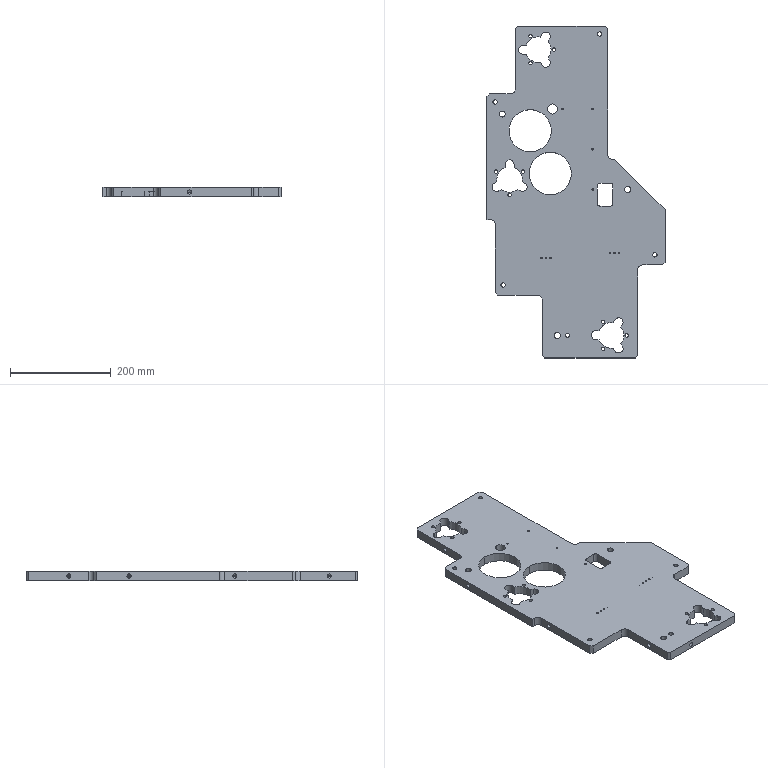Part | 1 solid | 698 faces | box 354 x 660 x 18 mm | volume 2444150 mm3 | cylinder 368 | cone 274 | plane 56 | commonest cylinder face diameters 3.3 x168 4 x58 4.2 x34 8.5 x28 6.8 x18 18 x13